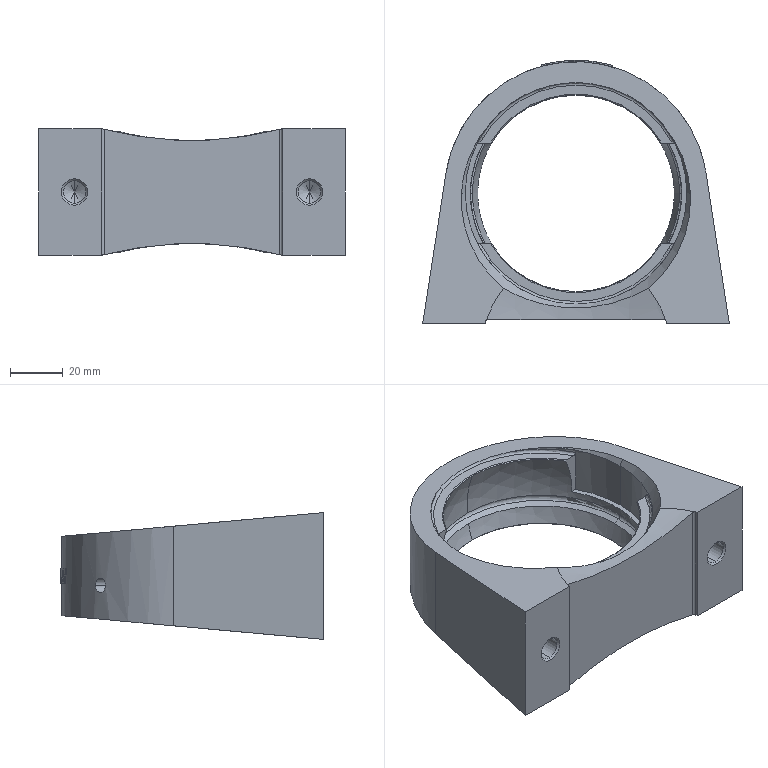Part | SolidWorks | features BaseBody 1 | 1 solid | 194 faces | box 116 x 99.5 x 48 mm | volume 160162 mm3 | plane 83 | cylinder 72 | cone 23 | torus 12 | sphere 4 | commonest cylinder face diameters 0.193 x14 0.333 x14 0.615 x13 0.189 x10 83.871 x6 8.5 x4